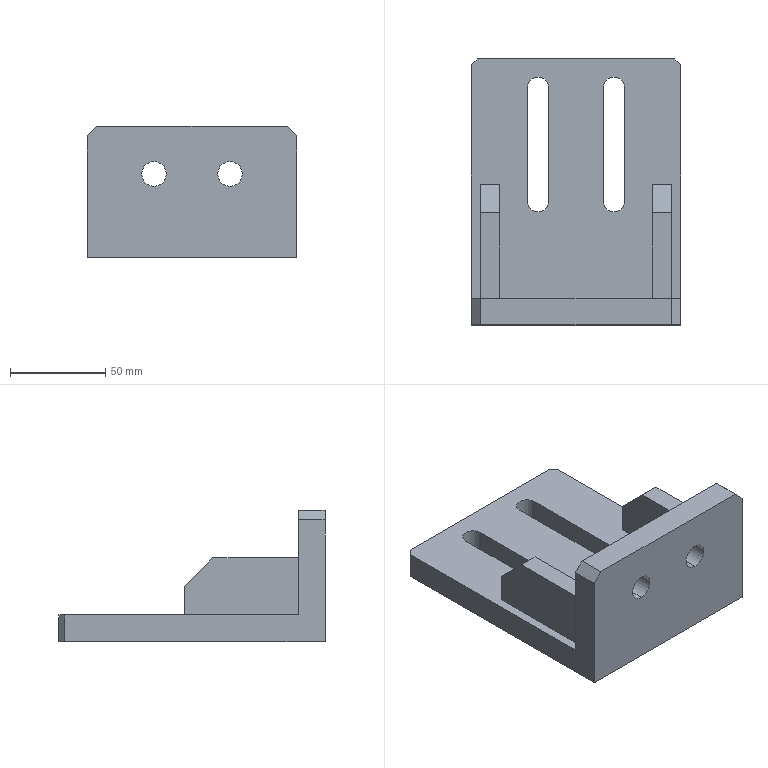Part | STEP file | Fixed Foot Plate | 1 solid | 34 faces | box 110 x 140 x 69 mm | volume 308717 mm3 | plane 26 | cylinder 8 | commonest cylinder face diameters 11 x4 13 x4